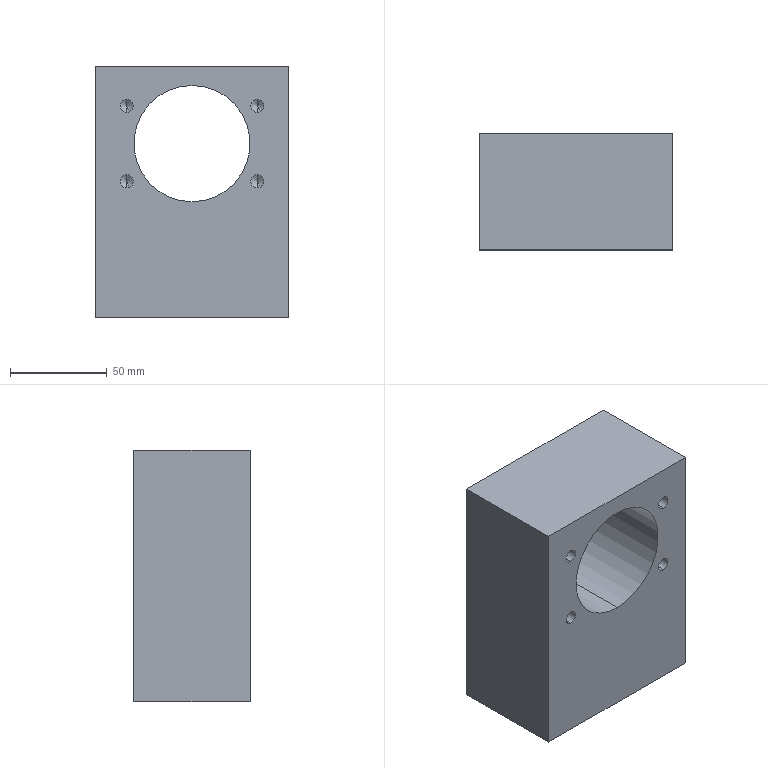Part | STEP file | 0244_204_Block | 1 solid | 40 faces | box 100 x 60 x 130 mm | volume 602094 mm3 | cylinder 18 | cone 16 | plane 6 | commonest cylinder face diameters 6.8 x16 60 x2